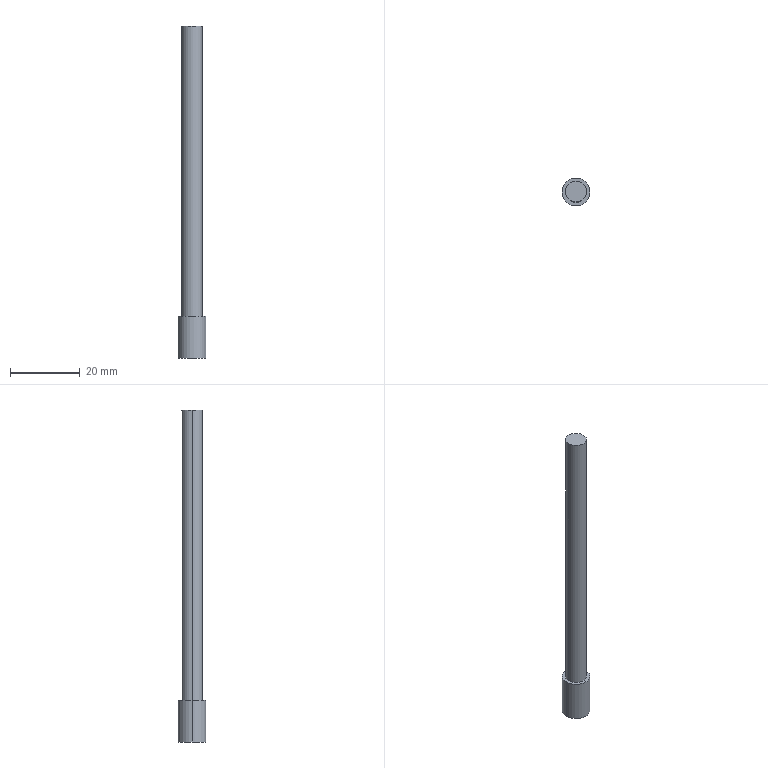Part | SolidWorks | features Extrusion 1, ICE 1 | 1 solid | 7 faces | box 8 x 8 x 95 mm | volume 2950 mm3 | cylinder 4 | plane 3 | commonest cylinder face diameters 6 x2 8 x2
STEP:
#1=CARTESIAN_POINT('',(3.,0.,12.));
#2=VERTEX_POINT('',#1);
#3=CARTESIAN_POINT('',(-3.,0.,12.));
#4=VERTEX_POINT('',#3);
#5=CARTESIAN_POINT('',(0.,0.,12.));
#6=DIRECTION('',(0.,0.,1.));
#7=DIRECTION('',(1.,0.,0.));
#8=AXIS2_PLACEMENT_3D('',#5,#6,#7);
#9=CIRCLE('',#8,3.);
#10=EDGE_CURVE('',#2,#4,#9,.T.);
#11=ORIENTED_EDGE('',*,*,#10,.T.);
#12=CARTESIAN_POINT('',(-3.,0.,95.));
#13=VERTEX_POINT('',#12);
#14=CARTESIAN_POINT('',(-3.,0.,12.));
#15=DIRECTION('',(0.,0.,1.));
#16=VECTOR('',#15,1000.);
#17=LINE('',#14,#16);
#18=EDGE_CURVE('',#4,#13,#17,.T.);
#19=ORIENTED_EDGE('',*,*,#18,.T.);
#20=CARTESIAN_POINT('',(3.,0.,95.));
#21=VERTEX_POINT('',#20);
#22=CARTESIAN_POINT('',(0.,0.,95.));
#23=DIRECTION('',(0.,0.,1.));
#24=DIRECTION('',(1.,0.,0.));
#25=AXIS2_PLACEMENT_3D('',#22,#23,#24);
#26=CIRCLE('',#25,3.);
#27=EDGE_CURVE('',#21,#13,#26,.T.);
#28=ORIENTED_EDGE('',*,*,#27,.F.);
#29=CARTESIAN_POINT('',(3.,0.,12.));
#30=DIRECTION('',(0.,0.,1.));
#31=VECTOR('',#30,1000.);
#32=LINE('',#29,#31);
#33=EDGE_CURVE('',#2,#21,#32,.T.);
#34=ORIENTED_EDGE('',*,*,#33,.F.);
#35=EDGE_LOOP('',(#11,#19,#28,#34));
#36=FACE_OUTER_BOUND('',#35,.T.);
#37=CARTESIAN_POINT('',(0.,0.,12.));
#38=DIRECTION('',(0.,0.,1.));
#39=DIRECTION('',(1.,0.,0.));
#40=AXIS2_PLACEMENT_3D('',#37,#38,#39);
#41=CYLINDRICAL_SURFACE('',#40,3.);
#42=ADVANCED_FACE('',(#36),#41,.T.);
#43=CARTESIAN_POINT('',(4.,0.,12.));
#44=VERTEX_POINT('',#43);
#45=CARTESIAN_POINT('',(-4.,0.,12.));
#46=VERTEX_POINT('',#45);
#47=CARTESIAN_POINT('',(0.,0.,12.));
#48=DIRECTION('',(0.,0.,1.));
#49=DIRECTION('',(1.,0.,0.));
#50=AXIS2_PLACEMENT_3D('',#47,#48,#49);
#51=CIRCLE('',#50,4.);
#52=EDGE_CURVE('',#44,#46,#51,.T.);
#53=ORIENTED_EDGE('',*,*,#52,.F.);
#54=CARTESIAN_POINT('',(4.,0.,0.));
#55=VERTEX_POINT('',#54);
#56=CARTESIAN_POINT('',(4.,0.,95.));
#57=DIRECTION('',(0.,0.,-1.));
#58=VECTOR('',#57,1000.);
#59=LINE('',#56,#58);
#60=EDGE_CURVE('',#44,#55,#59,.T.);
#61=ORIENTED_EDGE('',*,*,#60,.T.);
#62=CARTESIAN_POINT('',(-4.,0.,0.));
#63=VERTEX_POINT('',#62);
#64=CARTESIAN_POINT('',(0.,0.,0.));
#65=DIRECTION('',(0.,0.,1.));
#66=DIRECTION('',(1.,0.,0.));
#67=AXIS2_PLACEMENT_3D('',#64,#65,#66);
#68=CIRCLE('',#67,4.);
#69=EDGE_CURVE('',#55,#63,#68,.T.);
#70=ORIENTED_EDGE('',*,*,#69,.T.);
#71=CARTESIAN_POINT('',(-4.,0.,95.));
#72=DIRECTION('',(0.,0.,-1.));
#73=VECTOR('',#72,1000.);
#74=LINE('',#71,#73);
#75=EDGE_CURVE('',#46,#63,#74,.T.);
#76=ORIENTED_EDGE('',*,*,#75,.F.);
#77=EDGE_LOOP('',(#53,#61,#70,#76));
#78=FACE_OUTER_BOUND('',#77,.T.);
#79=CARTESIAN_POINT('',(0.,0.,95.));
#80=DIRECTION('',(0.,0.,-1.));
#81=DIRECTION('',(-1.,0.,0.));
#82=AXIS2_PLACEMENT_3D('',#79,#80,#81);
#83=CYLINDRICAL_SURFACE('',#82,4.);
#84=ADVANCED_FACE('',(#78),#83,.T.);
#85=ORIENTED_EDGE('',*,*,#60,.F.);
#86=CARTESIAN_POINT('',(0.,0.,12.));
#87=DIRECTION('',(0.,0.,1.));
#88=DIRECTION('',(1.,0.,0.));
#89=AXIS2_PLACEMENT_3D('',#86,#87,#88);
#90=CIRCLE('',#89,4.);
#91=EDGE_CURVE('',#46,#44,#90,.T.);
#92=ORIENTED_EDGE('',*,*,#91,.F.);
#93=ORIENTED_EDGE('',*,*,#75,.T.);
#94=CARTESIAN_POINT('',(0.,0.,0.));
#95=DIRECTION('',(0.,0.,1.));
#96=DIRECTION('',(1.,0.,0.));
#97=AXIS2_PLACEMENT_3D('',#94,#95,#96);
#98=CIRCLE('',#97,4.);
#99=EDGE_CURVE('',#63,#55,#98,.T.);
#100=ORIENTED_EDGE('',*,*,#99,.T.);
#101=EDGE_LOOP('',(#85,#92,#93,#100));
#102=FACE_OUTER_BOUND('',#101,.T.);
#103=CARTESIAN_POINT('',(0.,0.,95.));
#104=DIRECTION('',(0.,0.,-1.));
#105=DIRECTION('',(-1.,0.,0.));
#106=AXIS2_PLACEMENT_3D('',#103,#104,#105);
#107=CYLINDRICAL_SURFACE('',#106,4.);
#108=ADVANCED_FACE('',(#102),#107,.T.);
#109=ORIENTED_EDGE('',*,*,#99,.F.);
#110=ORIENTED_EDGE('',*,*,#69,.F.);
#111=EDGE_LOOP('',(#109,#110));
#112=FACE_OUTER_BOUND('',#111,.T.);
#113=CARTESIAN_POINT('',(0.,0.,0.));
#114=DIRECTION('',(0.,0.,1.));
#115=DIRECTION('',(1.,0.,0.));
#116=AXIS2_PLACEMENT_3D('',#113,#114,#115);
#117=PLANE('',#116);
#118=ADVANCED_FACE('',(#112),#117,.F.);
#119=ORIENTED_EDGE('',*,*,#10,.F.);
#120=CARTESIAN_POINT('',(0.,0.,12.));
#121=DIRECTION('',(0.,0.,1.));
#122=DIRECTION('',(1.,0.,0.));
#123=AXIS2_PLACEMENT_3D('',#120,#121,#122);
#124=CIRCLE('',#123,3.);
#125=EDGE_CURVE('',#4,#2,#124,.T.);
#126=ORIENTED_EDGE('',*,*,#125,.F.);
#127=EDGE_LOOP('',(#119,#126));
#128=FACE_BOUND('',#127,.T.);
#129=ORIENTED_EDGE('',*,*,#91,.T.);
#130=ORIENTED_EDGE('',*,*,#52,.T.);
#131=EDGE_LOOP('',(#129,#130));
#132=FACE_OUTER_BOUND('',#131,.T.);
#133=CARTESIAN_POINT('',(0.,0.,12.));
#134=DIRECTION('',(0.,0.,1.));
#135=DIRECTION('',(1.,0.,0.));
#136=AXIS2_PLACEMENT_3D('',#133,#134,#135);
#137=PLANE('',#136);
#138=ADVANCED_FACE('',(#128,#132),#137,.T.);
#139=ORIENTED_EDGE('',*,*,#18,.F.);
#140=ORIENTED_EDGE('',*,*,#125,.T.);
#141=ORIENTED_EDGE('',*,*,#33,.T.);
#142=CARTESIAN_POINT('',(0.,0.,95.));
#143=DIRECTION('',(0.,0.,1.));
#144=DIRECTION('',(1.,0.,0.));
#145=AXIS2_PLACEMENT_3D('',#142,#143,#144);
#146=CIRCLE('',#145,3.);
#147=EDGE_CURVE('',#13,#21,#146,.T.);
#148=ORIENTED_EDGE('',*,*,#147,.F.);
#149=EDGE_LOOP('',(#139,#140,#141,#148));
#150=FACE_OUTER_BOUND('',#149,.T.);
#151=CARTESIAN_POINT('',(0.,0.,12.));
#152=DIRECTION('',(0.,0.,1.));
#153=DIRECTION('',(1.,0.,0.));
#154=AXIS2_PLACEMENT_3D('',#151,#152,#153);
#155=CYLINDRICAL_SURFACE('',#154,3.);
#156=ADVANCED_FACE('',(#150),#155,.T.);
#157=ORIENTED_EDGE('',*,*,#27,.T.);
#158=ORIENTED_EDGE('',*,*,#147,.T.);
#159=EDGE_LOOP('',(#157,#158));
#160=FACE_OUTER_BOUND('',#159,.T.);
#161=CARTESIAN_POINT('',(0.,0.,95.));
#162=DIRECTION('',(0.,0.,1.));
#163=DIRECTION('',(1.,0.,0.));
#164=AXIS2_PLACEMENT_3D('',#161,#162,#163);
#165=PLANE('',#164);
#166=ADVANCED_FACE('',(#160),#165,.T.);
#167=CLOSED_SHELL('',(#42,#84,#108,#118,#138,#156,#166));
#168=MANIFOLD_SOLID_BREP('',#167);
#169=CARTESIAN_POINT('',(0.,0.,0.));
#170=DIRECTION('',(0.,0.,1.));
#171=DIRECTION('',(1.,0.,0.));
#172=AXIS2_PLACEMENT_3D('',#169,#170,#171);
#173=(LENGTH_UNIT()NAMED_UNIT(*)SI_UNIT(.MILLI.,.METRE.));
#174=UNCERTAINTY_MEASURE_WITH_UNIT(LENGTH_MEASURE(0.00001),#173,'','');
#175=(NAMED_UNIT(*)PLANE_ANGLE_UNIT()SI_UNIT($,.RADIAN.));
#176=(NAMED_UNIT(*)SI_UNIT($,.STERADIAN.)SOLID_ANGLE_UNIT());
#177=(GEOMETRIC_REPRESENTATION_CONTEXT(3)GLOBAL_UNCERTAINTY_ASSIGNED_CONTEXT((#174))GLOBAL_UNIT_ASSIGNED_CONTEXT((#173,#175,#176))REPRESENTATION_CONTEXT('',''));
#178=ADVANCED_BREP_SHAPE_REPRESENTATION('',(#168,#172),#177);